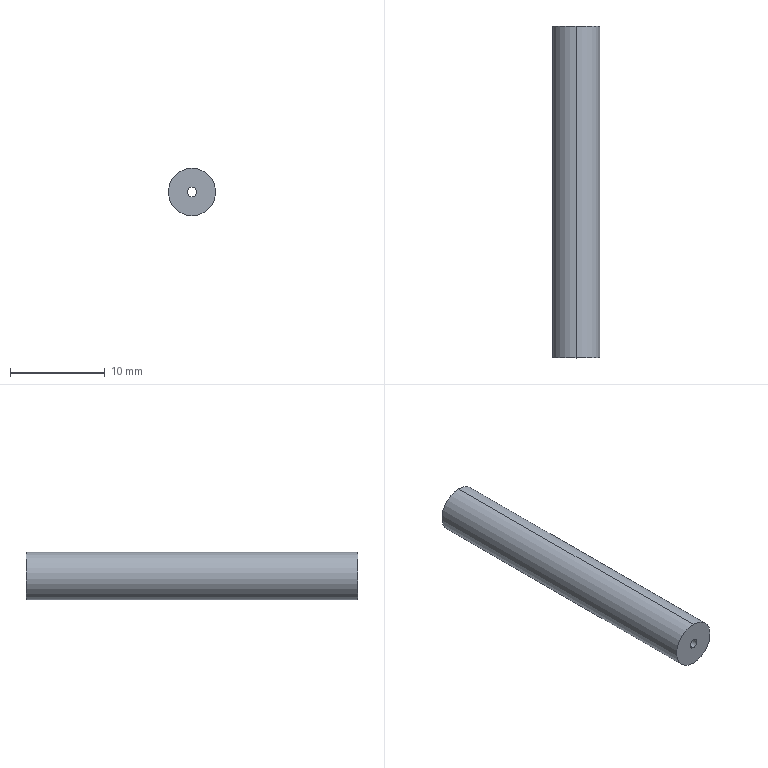Part | SolidWorks | features Extrusion 1, ICE 1 | 1 solid | 9 faces | box 5 x 35 x 5 mm | volume 452.389 mm3 | cylinder 6 | plane 3 | commonest cylinder face diameters 1 x2 3 x2 5 x2
STEP:
#1=CARTESIAN_POINT('',(0.,2.,0.5));
#2=VERTEX_POINT('',#1);
#3=CARTESIAN_POINT('',(0.,2.,-0.5));
#4=VERTEX_POINT('',#3);
#5=CARTESIAN_POINT('',(0.,2.,0.));
#6=DIRECTION('',(0.,-1.,0.));
#7=DIRECTION('',(0.,0.,-1.));
#8=AXIS2_PLACEMENT_3D('',#5,#6,#7);
#9=CIRCLE('',#8,0.5);
#10=EDGE_CURVE('',#2,#4,#9,.T.);
#11=ORIENTED_EDGE('',*,*,#10,.F.);
#12=CARTESIAN_POINT('',(0.,0.,0.5));
#13=VERTEX_POINT('',#12);
#14=CARTESIAN_POINT('',(0.,2.,0.5));
#15=DIRECTION('',(0.,-1.,0.));
#16=VECTOR('',#15,1000.);
#17=LINE('',#14,#16);
#18=EDGE_CURVE('',#2,#13,#17,.T.);
#19=ORIENTED_EDGE('',*,*,#18,.T.);
#20=CARTESIAN_POINT('',(0.,0.,-0.5));
#21=VERTEX_POINT('',#20);
#22=CARTESIAN_POINT('',(0.,0.,0.));
#23=DIRECTION('',(0.,-1.,0.));
#24=DIRECTION('',(0.,0.,-1.));
#25=AXIS2_PLACEMENT_3D('',#22,#23,#24);
#26=CIRCLE('',#25,0.5);
#27=EDGE_CURVE('',#13,#21,#26,.T.);
#28=ORIENTED_EDGE('',*,*,#27,.T.);
#29=CARTESIAN_POINT('',(0.,2.,-0.5));
#30=DIRECTION('',(0.,-1.,0.));
#31=VECTOR('',#30,1000.);
#32=LINE('',#29,#31);
#33=EDGE_CURVE('',#4,#21,#32,.T.);
#34=ORIENTED_EDGE('',*,*,#33,.F.);
#35=EDGE_LOOP('',(#11,#19,#28,#34));
#36=FACE_OUTER_BOUND('',#35,.T.);
#37=CARTESIAN_POINT('',(0.,2.,0.));
#38=DIRECTION('',(0.,-1.,0.));
#39=DIRECTION('',(0.,0.,-1.));
#40=AXIS2_PLACEMENT_3D('',#37,#38,#39);
#41=CYLINDRICAL_SURFACE('',#40,0.5);
#42=ADVANCED_FACE('',(#36),#41,.F.);
#43=CARTESIAN_POINT('',(0.,35.,2.5));
#44=VERTEX_POINT('',#43);
#45=CARTESIAN_POINT('',(0.,35.,-2.5));
#46=VERTEX_POINT('',#45);
#47=CARTESIAN_POINT('',(0.,35.,0.));
#48=DIRECTION('',(0.,1.,0.));
#49=DIRECTION('',(0.,0.,1.));
#50=AXIS2_PLACEMENT_3D('',#47,#48,#49);
#51=CIRCLE('',#50,2.5);
#52=EDGE_CURVE('',#44,#46,#51,.T.);
#53=ORIENTED_EDGE('',*,*,#52,.F.);
#54=CARTESIAN_POINT('',(0.,0.,2.5));
#55=VERTEX_POINT('',#54);
#56=CARTESIAN_POINT('',(0.,35.,2.5));
#57=DIRECTION('',(0.,-1.,0.));
#58=VECTOR('',#57,1000.);
#59=LINE('',#56,#58);
#60=EDGE_CURVE('',#44,#55,#59,.T.);
#61=ORIENTED_EDGE('',*,*,#60,.T.);
#62=CARTESIAN_POINT('',(0.,0.,-2.5));
#63=VERTEX_POINT('',#62);
#64=CARTESIAN_POINT('',(0.,0.,0.));
#65=DIRECTION('',(0.,1.,0.));
#66=DIRECTION('',(0.,0.,1.));
#67=AXIS2_PLACEMENT_3D('',#64,#65,#66);
#68=CIRCLE('',#67,2.5);
#69=EDGE_CURVE('',#55,#63,#68,.T.);
#70=ORIENTED_EDGE('',*,*,#69,.T.);
#71=CARTESIAN_POINT('',(0.,35.,-2.5));
#72=DIRECTION('',(0.,-1.,0.));
#73=VECTOR('',#72,1000.);
#74=LINE('',#71,#73);
#75=EDGE_CURVE('',#46,#63,#74,.T.);
#76=ORIENTED_EDGE('',*,*,#75,.F.);
#77=EDGE_LOOP('',(#53,#61,#70,#76));
#78=FACE_OUTER_BOUND('',#77,.T.);
#79=CARTESIAN_POINT('',(0.,35.,0.));
#80=DIRECTION('',(0.,-1.,0.));
#81=DIRECTION('',(0.,0.,-1.));
#82=AXIS2_PLACEMENT_3D('',#79,#80,#81);
#83=CYLINDRICAL_SURFACE('',#82,2.5);
#84=ADVANCED_FACE('',(#78),#83,.T.);
#85=CARTESIAN_POINT('',(0.,35.,-1.5));
#86=VERTEX_POINT('',#85);
#87=CARTESIAN_POINT('',(0.,35.,1.5));
#88=VERTEX_POINT('',#87);
#89=CARTESIAN_POINT('',(0.,35.,0.));
#90=DIRECTION('',(0.,1.,0.));
#91=DIRECTION('',(0.,0.,1.));
#92=AXIS2_PLACEMENT_3D('',#89,#90,#91);
#93=CIRCLE('',#92,1.5);
#94=EDGE_CURVE('',#86,#88,#93,.T.);
#95=ORIENTED_EDGE('',*,*,#94,.T.);
#96=CARTESIAN_POINT('',(0.,2.,1.5));
#97=VERTEX_POINT('',#96);
#98=CARTESIAN_POINT('',(0.,35.,1.5));
#99=DIRECTION('',(0.,-1.,0.));
#100=VECTOR('',#99,1000.);
#101=LINE('',#98,#100);
#102=EDGE_CURVE('',#88,#97,#101,.T.);
#103=ORIENTED_EDGE('',*,*,#102,.T.);
#104=CARTESIAN_POINT('',(0.,2.,-1.5));
#105=VERTEX_POINT('',#104);
#106=CARTESIAN_POINT('',(0.,2.,0.));
#107=DIRECTION('',(0.,-1.,0.));
#108=DIRECTION('',(0.,0.,-1.));
#109=AXIS2_PLACEMENT_3D('',#106,#107,#108);
#110=CIRCLE('',#109,1.5);
#111=EDGE_CURVE('',#97,#105,#110,.T.);
#112=ORIENTED_EDGE('',*,*,#111,.T.);
#113=CARTESIAN_POINT('',(0.,35.,-1.5));
#114=DIRECTION('',(0.,-1.,0.));
#115=VECTOR('',#114,1000.);
#116=LINE('',#113,#115);
#117=EDGE_CURVE('',#86,#105,#116,.T.);
#118=ORIENTED_EDGE('',*,*,#117,.F.);
#119=EDGE_LOOP('',(#95,#103,#112,#118));
#120=FACE_OUTER_BOUND('',#119,.T.);
#121=CARTESIAN_POINT('',(0.,35.,0.));
#122=DIRECTION('',(0.,-1.,0.));
#123=DIRECTION('',(0.,0.,-1.));
#124=AXIS2_PLACEMENT_3D('',#121,#122,#123);
#125=CYLINDRICAL_SURFACE('',#124,1.5);
#126=ADVANCED_FACE('',(#120),#125,.F.);
#127=ORIENTED_EDGE('',*,*,#102,.F.);
#128=CARTESIAN_POINT('',(0.,35.,0.));
#129=DIRECTION('',(0.,1.,0.));
#130=DIRECTION('',(0.,0.,1.));
#131=AXIS2_PLACEMENT_3D('',#128,#129,#130);
#132=CIRCLE('',#131,1.5);
#133=EDGE_CURVE('',#88,#86,#132,.T.);
#134=ORIENTED_EDGE('',*,*,#133,.T.);
#135=ORIENTED_EDGE('',*,*,#117,.T.);
#136=CARTESIAN_POINT('',(0.,2.,0.));
#137=DIRECTION('',(0.,-1.,0.));
#138=DIRECTION('',(0.,0.,-1.));
#139=AXIS2_PLACEMENT_3D('',#136,#137,#138);
#140=CIRCLE('',#139,1.5);
#141=EDGE_CURVE('',#105,#97,#140,.T.);
#142=ORIENTED_EDGE('',*,*,#141,.T.);
#143=EDGE_LOOP('',(#127,#134,#135,#142));
#144=FACE_OUTER_BOUND('',#143,.T.);
#145=CARTESIAN_POINT('',(0.,35.,0.));
#146=DIRECTION('',(0.,-1.,0.));
#147=DIRECTION('',(0.,0.,-1.));
#148=AXIS2_PLACEMENT_3D('',#145,#146,#147);
#149=CYLINDRICAL_SURFACE('',#148,1.5);
#150=ADVANCED_FACE('',(#144),#149,.F.);
#151=CARTESIAN_POINT('',(0.,35.,0.));
#152=DIRECTION('',(0.,1.,0.));
#153=DIRECTION('',(0.,0.,1.));
#154=AXIS2_PLACEMENT_3D('',#151,#152,#153);
#155=CIRCLE('',#154,2.5);
#156=EDGE_CURVE('',#46,#44,#155,.T.);
#157=ORIENTED_EDGE('',*,*,#156,.T.);
#158=ORIENTED_EDGE('',*,*,#52,.T.);
#159=EDGE_LOOP('',(#157,#158));
#160=FACE_OUTER_BOUND('',#159,.T.);
#161=ORIENTED_EDGE('',*,*,#94,.F.);
#162=ORIENTED_EDGE('',*,*,#133,.F.);
#163=EDGE_LOOP('',(#161,#162));
#164=FACE_BOUND('',#163,.T.);
#165=CARTESIAN_POINT('',(0.,35.,0.));
#166=DIRECTION('',(0.,1.,0.));
#167=DIRECTION('',(0.,0.,1.));
#168=AXIS2_PLACEMENT_3D('',#165,#166,#167);
#169=PLANE('',#168);
#170=ADVANCED_FACE('',(#160,#164),#169,.T.);
#171=CARTESIAN_POINT('',(0.,0.,0.));
#172=DIRECTION('',(0.,1.,0.));
#173=DIRECTION('',(0.,0.,1.));
#174=AXIS2_PLACEMENT_3D('',#171,#172,#173);
#175=CIRCLE('',#174,2.5);
#176=EDGE_CURVE('',#63,#55,#175,.T.);
#177=ORIENTED_EDGE('',*,*,#176,.F.);
#178=ORIENTED_EDGE('',*,*,#69,.F.);
#179=EDGE_LOOP('',(#177,#178));
#180=FACE_OUTER_BOUND('',#179,.T.);
#181=CARTESIAN_POINT('',(0.,0.,0.));
#182=DIRECTION('',(0.,-1.,0.));
#183=DIRECTION('',(0.,0.,-1.));
#184=AXIS2_PLACEMENT_3D('',#181,#182,#183);
#185=CIRCLE('',#184,0.5);
#186=EDGE_CURVE('',#21,#13,#185,.T.);
#187=ORIENTED_EDGE('',*,*,#186,.F.);
#188=ORIENTED_EDGE('',*,*,#27,.F.);
#189=EDGE_LOOP('',(#187,#188));
#190=FACE_BOUND('',#189,.T.);
#191=CARTESIAN_POINT('',(0.,0.,0.));
#192=DIRECTION('',(0.,1.,0.));
#193=DIRECTION('',(0.,0.,1.));
#194=AXIS2_PLACEMENT_3D('',#191,#192,#193);
#195=PLANE('',#194);
#196=ADVANCED_FACE('',(#180,#190),#195,.F.);
#197=ORIENTED_EDGE('',*,*,#60,.F.);
#198=ORIENTED_EDGE('',*,*,#156,.F.);
#199=ORIENTED_EDGE('',*,*,#75,.T.);
#200=ORIENTED_EDGE('',*,*,#176,.T.);
#201=EDGE_LOOP('',(#197,#198,#199,#200));
#202=FACE_OUTER_BOUND('',#201,.T.);
#203=CARTESIAN_POINT('',(0.,35.,0.));
#204=DIRECTION('',(0.,-1.,0.));
#205=DIRECTION('',(0.,0.,-1.));
#206=AXIS2_PLACEMENT_3D('',#203,#204,#205);
#207=CYLINDRICAL_SURFACE('',#206,2.5);
#208=ADVANCED_FACE('',(#202),#207,.T.);
#209=CARTESIAN_POINT('',(0.,2.,0.));
#210=DIRECTION('',(0.,-1.,0.));
#211=DIRECTION('',(0.,0.,-1.));
#212=AXIS2_PLACEMENT_3D('',#209,#210,#211);
#213=CIRCLE('',#212,0.5);
#214=EDGE_CURVE('',#4,#2,#213,.T.);
#215=ORIENTED_EDGE('',*,*,#214,.T.);
#216=ORIENTED_EDGE('',*,*,#10,.T.);
#217=EDGE_LOOP('',(#215,#216));
#218=FACE_BOUND('',#217,.T.);
#219=ORIENTED_EDGE('',*,*,#141,.F.);
#220=ORIENTED_EDGE('',*,*,#111,.F.);
#221=EDGE_LOOP('',(#219,#220));
#222=FACE_OUTER_BOUND('',#221,.T.);
#223=CARTESIAN_POINT('',(0.,2.,0.));
#224=DIRECTION('',(0.,-1.,0.));
#225=DIRECTION('',(0.,0.,-1.));
#226=AXIS2_PLACEMENT_3D('',#223,#224,#225);
#227=PLANE('',#226);
#228=ADVANCED_FACE('',(#218,#222),#227,.F.);
#229=ORIENTED_EDGE('',*,*,#18,.F.);
#230=ORIENTED_EDGE('',*,*,#214,.F.);
#231=ORIENTED_EDGE('',*,*,#33,.T.);
#232=ORIENTED_EDGE('',*,*,#186,.T.);
#233=EDGE_LOOP('',(#229,#230,#231,#232));
#234=FACE_OUTER_BOUND('',#233,.T.);
#235=CARTESIAN_POINT('',(0.,2.,0.));
#236=DIRECTION('',(0.,-1.,0.));
#237=DIRECTION('',(0.,0.,-1.));
#238=AXIS2_PLACEMENT_3D('',#235,#236,#237);
#239=CYLINDRICAL_SURFACE('',#238,0.5);
#240=ADVANCED_FACE('',(#234),#239,.F.);
#241=CLOSED_SHELL('',(#42,#84,#126,#150,#170,#196,#208,#228,#240));
#242=MANIFOLD_SOLID_BREP('',#241);
#243=CARTESIAN_POINT('',(0.,0.,0.));
#244=DIRECTION('',(0.,0.,1.));
#245=DIRECTION('',(1.,0.,0.));
#246=AXIS2_PLACEMENT_3D('',#243,#244,#245);
#247=(LENGTH_UNIT()NAMED_UNIT(*)SI_UNIT(.MILLI.,.METRE.));
#248=UNCERTAINTY_MEASURE_WITH_UNIT(LENGTH_MEASURE(0.00001),#247,'','');
#249=(NAMED_UNIT(*)PLANE_ANGLE_UNIT()SI_UNIT($,.RADIAN.));
#250=(NAMED_UNIT(*)SI_UNIT($,.STERADIAN.)SOLID_ANGLE_UNIT());
#251=(GEOMETRIC_REPRESENTATION_CONTEXT(3)GLOBAL_UNCERTAINTY_ASSIGNED_CONTEXT((#248))GLOBAL_UNIT_ASSIGNED_CONTEXT((#247,#249,#250))REPRESENTATION_CONTEXT('',''));
#252=ADVANCED_BREP_SHAPE_REPRESENTATION('',(#242,#246),#251);